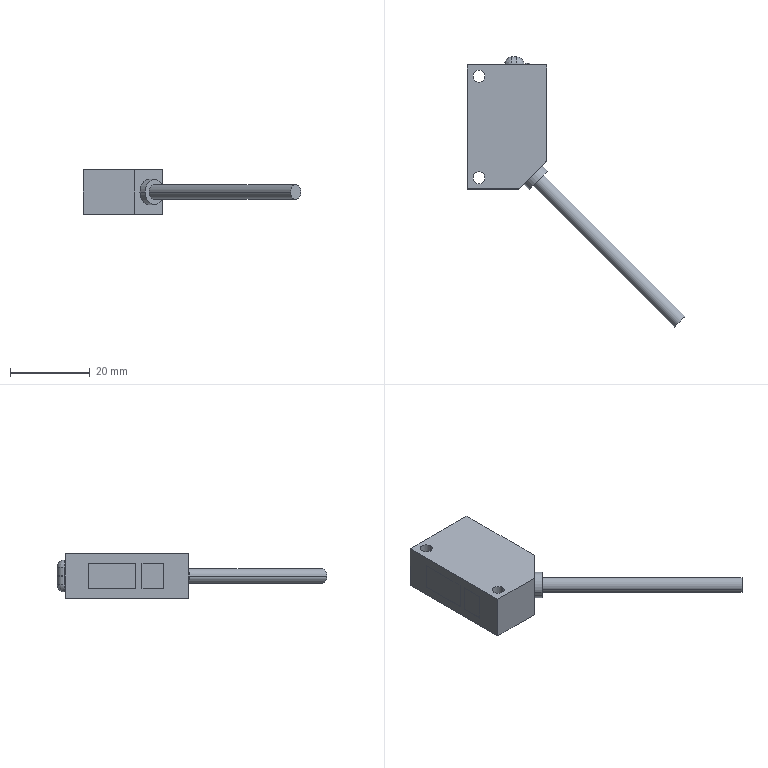Part | SolidWorks | features BaseBody 3 | 3 solids | 110 faces | box 54.507 x 67.507 x 11.2 mm | volume 7170 mm3 | plane 69 | cylinder 37 | spline 4 | commonest cylinder face diameters 3.6 x10 2.2 x9 0.4 x5 3 x4 4.1 x3 3.4 x2